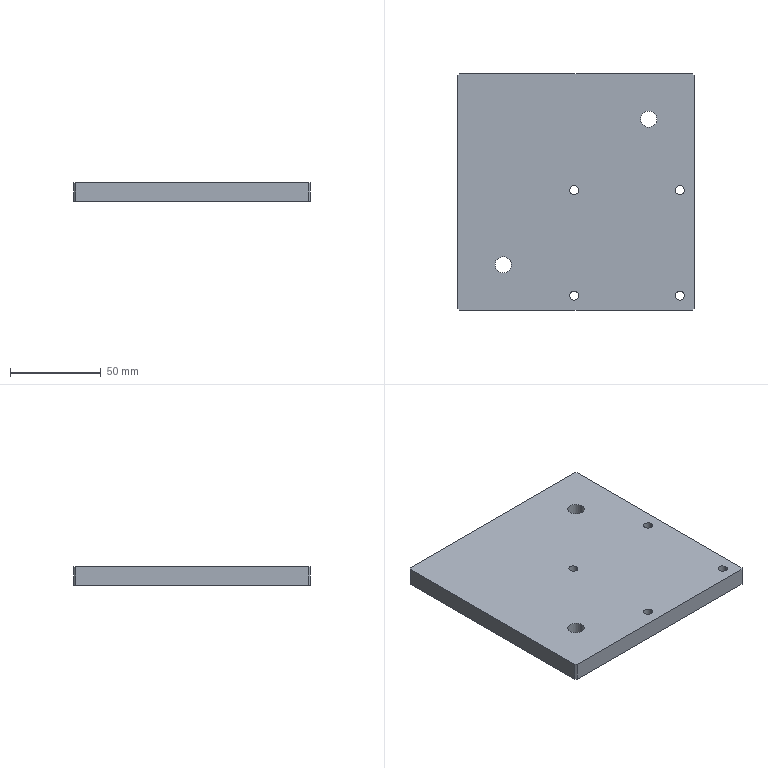Part | STEP file | Foot plate 2 | 1 solid | 22 faces | box 130 x 130 x 10 mm | volume 166922 mm3 | cylinder 12 | plane 10 | commonest cylinder face diameters 5 x8 9 x4